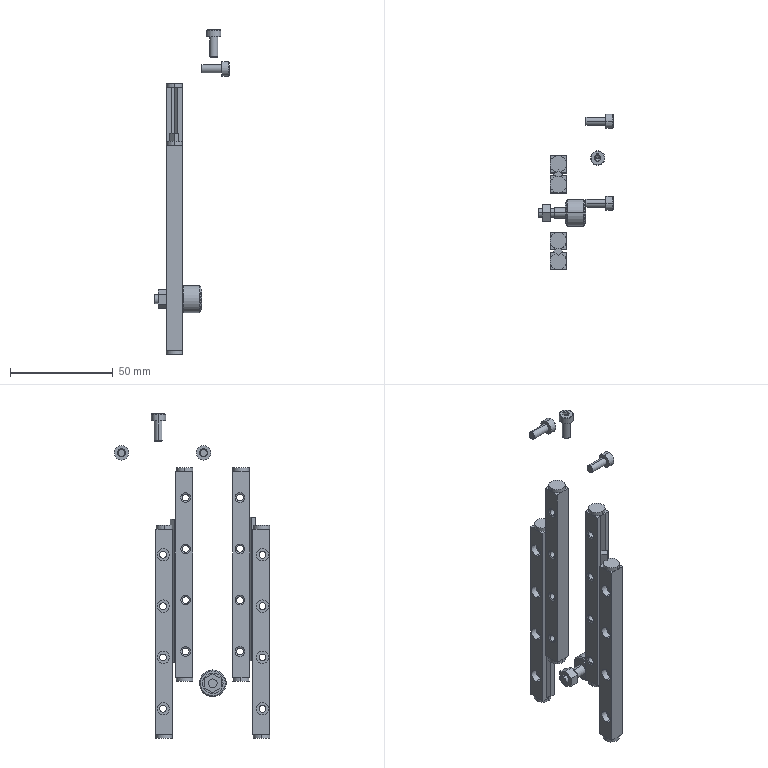Part | NX | 11 solids | 414 faces | box 36.3 x 75.7 x 158.36 mm | volume 28101 mm3 | plane 250 | cylinder 110 | cone 54 | commonest cylinder face diameters 3.3 x32 6 x32 8 x16 3 x6 4 x6 7 x6